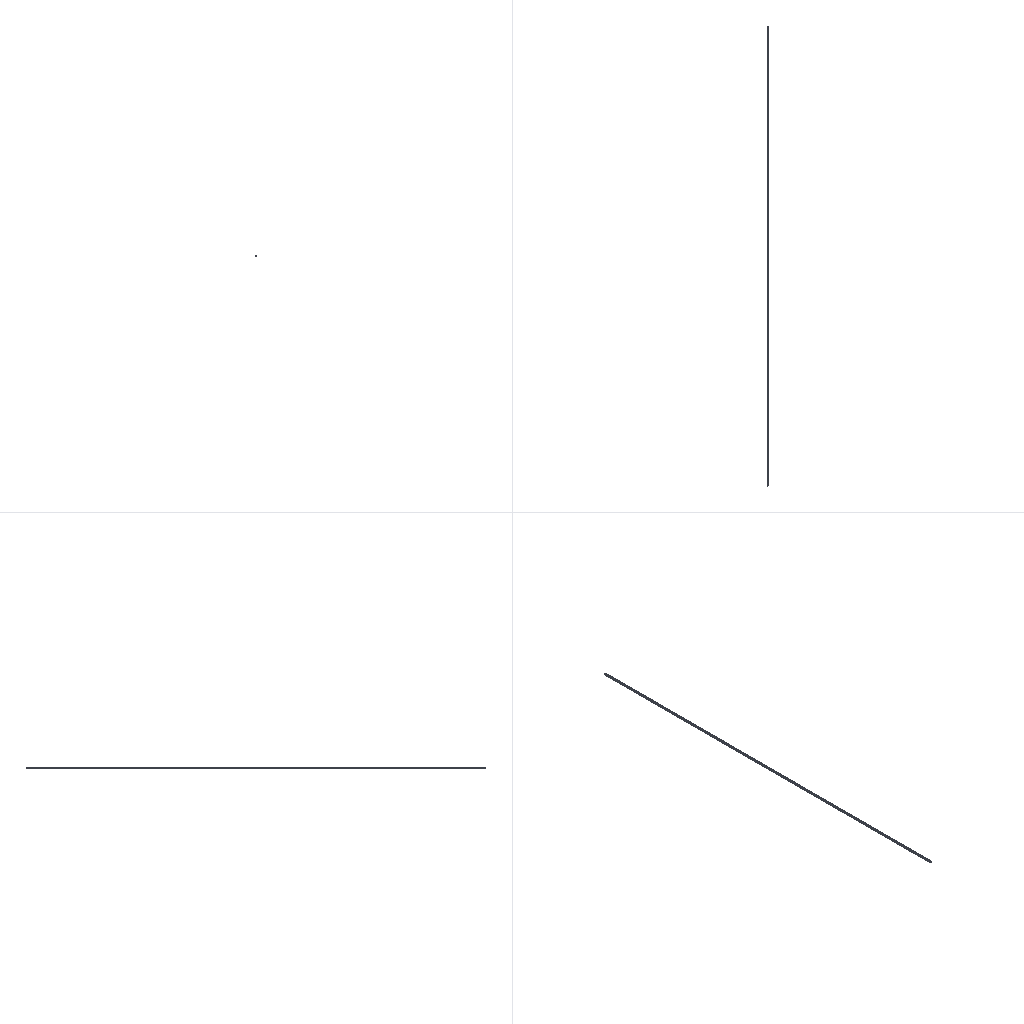Simulation study | abaqus
Set-up summary:
category,name,step,type,value,unit,region
solver,abaqus
solver,version,,,Abaqus/Explicit 2020
units,not stated in the deck,,not stated
analysis,deck,,transient,transient
load_step,Step-1,Step-1,transient
load_step,requested,,,1
mesh,nodes,,,19475
mesh,elements,,,19439
element_type,S4R,,shell,13455
element_type,R3D4,,rigid,5984
load,load commands in deck,,count,2
bc,support commands in deck,,count,1
material,MATERIAL-1,,in results
check,setup vs results,,match,"per instance, exact: element labels, types and connectivity; labels of the nodes the elements use; coordinates of those nodes at SINGLE_PRECISION in 2 of 2 instance(s)"
Abaqus input file, long lists of numbers shortened:
*Heading
** Job name: Job-1 Model name: Model-1
** Generated by: Abaqus/CAE 2020
*Preprint, echo=NO, model=NO, history=NO, contact=NO
**
** PARTS
**
*Part, name=rig
*Node
      1,         175.,  -1827.906,  -4.069
      2,          25.,  -1827.906,  -4.069
** (6004 more lines like these left out)
*Element, type=R3D4
   1,    1,    5,   89,  110
   2,    5,    6,   90,   89
** (5982 more lines like these left out)
*Node
   6007,   2.906,       -1800.,   4.069
*Nset, nset=rig-RefPt_, internal
6007,
*Elset, elset=rig, generate
    1,  5984,     1
*End Part
**
*Part, name=tube
*Node
      1, -0.01062,        -750., -0.9999
      2,  0.4553,        -750., -0.8903
** (13466 more lines like these left out)
*Element, type=S4R
    1,    13,     1,    14,    26
    2,     1,     2,    15,    14
** (13453 more lines like these left out)
*Nset, nset=Set-1, generate
     1,  13468,      1
*Elset, elset=Set-1, generate
     1,  13455,      1
** Section: Section-1
*Shell Section, elset=Set-1, material=Material-1
0.002, 5
*End Part
**
**
** ASSEMBLY
**
*Assembly, name=Assembly
**
*Instance, name=rig-1, part=rig
          0.,        1600.,           0.
*End Instance
**
*Instance, name=tube-1, part=tube
          0.,         550.,           0.
*End Instance
**
*Node
      1,           0.,         300., 6.12323426e-17
*Nset, nset=Set-1, instance=rig-1
 6007,
*Nset, nset=Set-2, instance=tube-1, generate
 13456,  13468,      1
*Elset, elset=Set-2, instance=tube-1, generate
 13443,  13455,      1
*Nset, nset=Set-3, instance=tube-1, generate
 13456,  13468,      1
*Elset, elset=Set-3, instance=tube-1, generate
 13443,  13455,      1
*Nset, nset=Set-4, instance=tube-1, generate
     1,  13468,      1
*Elset, elset=Set-4, instance=tube-1, generate
     1,  13455,      1
*Nset, nset=Set-6
 1,
*Nset, nset=Set-7, instance=tube-1, generate
     1,  13468,      1
*Elset, elset=Set-7, instance=tube-1, generate
     1,  13455,      1
*Nset, nset=Set-8, instance=tube-1, generate
     1,  13468,      1
*Elset, elset=Set-8, instance=tube-1, generate
     1,  13455,      1
*Nset, nset=Set-9, instance=tube-1, generate
 13456,  13468,      1
*Elset, elset=Set-9, instance=tube-1, generate
 13443,  13455,      1
*Nset, nset=Set-10, instance=tube-1, generate
     1,  13468,      1
*Elset, elset=Set-10, instance=tube-1, generate
     1,  13455,      1
*Nset, nset=m_Set-5
 1,
*Elset, elset=_Surf-2_E3, internal, instance=tube-1, generate
 13443,  13455,      1
*Surface, type=ELEMENT, name=Surf-2
_Surf-2_E3, E3
*Elset, elset=_Surf-3_E3, internal, instance=tube-1, generate
 13443,  13455,      1
*Surface, type=ELEMENT, name=Surf-3
_Surf-3_E3, E3
*Elset, elset=_Surf-10_SNEG, internal, instance=tube-1, generate
     1,  13455,      1
*Surface, type=ELEMENT, name=Surf-10
_Surf-10_SNEG, SNEG
*Elset, elset=_m_Surf-4_SPOS, internal, instance=rig-1, generate
 2905,  5984,     1
*Surface, type=ELEMENT, name=m_Surf-4
_m_Surf-4_SPOS, SPOS
*Elset, elset=_m_Surf-7_SPOS, internal, instance=rig-1, generate
    1,  5984,     1
*Surface, type=ELEMENT, name=m_Surf-7
_m_Surf-7_SPOS, SPOS
*Elset, elset=_m_Surf-8_SPOS, internal, instance=rig-1, generate
    1,  5984,     1
*Surface, type=ELEMENT, name=m_Surf-8
_m_Surf-8_SPOS, SPOS
*Elset, elset=_s_Surf-1_E3, internal, instance=tube-1, generate
 13443,  13455,      1
*Surface, type=ELEMENT, name=s_Surf-1
_s_Surf-1_E3, E3
*Elset, elset=_s_Surf-4_SNEG, internal, instance=tube-1, generate
     1,  13455,      1
*Surface, type=ELEMENT, name=s_Surf-4
_s_Surf-4_SNEG, SNEG
*Elset, elset=_s_Surf-8_SNEG, internal, instance=tube-1, generate
     1,  13455,      1
*Surface, type=ELEMENT, name=s_Surf-8
_s_Surf-8_SNEG, SNEG
*Rigid Body, ref node=rig-1.rig-RefPt_, elset=rig-1.rig
** Constraint: Constraint-1
*Coupling, constraint name=Constraint-1, ref node=m_Set-5, surface=s_Surf-1
*Kinematic
*End Assembly
*Amplitude, name=Amp-1
             0.,              0.,              1.,              1.
**
** MATERIALS
**
*Material, name=Material-1
*Density
7850.,
*Elastic
 2.1e+11, 0.3
**
** INTERACTION PROPERTIES
**
*Surface Interaction, name=IntProp-1
*Friction
 0.2,
*Surface Behavior, pressure-overclosure=HARD
**
** CONTACT INITIALIZATION DATA
**
*Contact Initialization Data, name=CInit-1, INITIAL CLEARANCE=1.
**
** INTERACTIONS
**
** Interaction: Int-4
*Contact, op=NEW
*Contact Inclusions, ALL EXTERIOR
*Contact Property Assignment
 ,  , IntProp-1
** ----------------------------------------------------------------
**
** STEP: Step-1
**
*Step, name=Step-1, nlgeom=YES
*Dynamic, Explicit
, 10.
*Bulk Viscosity
0.06, 1.2
**
** BOUNDARY CONDITIONS
**
** Name: BC-1 Type: 对称/反对称/完全固定
*Boundary
Set-1, ENCASTRE
**
** LOADS
**
** Name: Load-1   Type: Concentrated force
*Cload
Set-6, 2, -50.
** Name: Load-3   Type: Gravity
*Dload
Set-7, GRAV, 9.8, 0., -1., 0.
**
** OUTPUT REQUESTS
**
*Restart, write, number interval=1, time marks=NO
**
** FIELD OUTPUT: F-Output-1
**
*Output, field
*Node Output
CF, RF, U, V
*Element Output, directions=YES
E, LE, MISES, MISESMAX, PE, PEEQ, PEEQMAX, PEEQT, PEMAG, S, SSAVG
*Contact Output
CDISP, CSTRESS
**
** HISTORY OUTPUT: H-Output-1
**
*Output, history, variable=PRESELECT, frequency=1
*End Step
Results summary:
result,step,Step-1,completed,increments=133046 time=10.0/10.0
result,analysis,,,transient
result,last_loadstep,,,1
result,primary field,,,"U, UR"
result,reaction total,,FX,-112324.406,model units
result,reaction total,,FY,357100.844,model units
result,reaction total,,FZ,-23574.062,model units